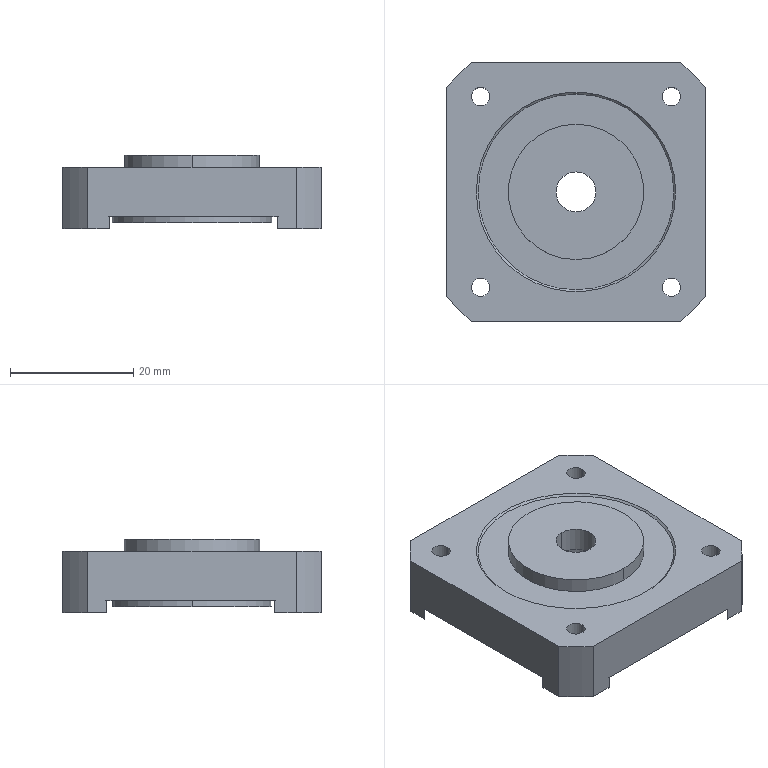Part | SolidWorks | features BaseBody 1 | 1 solid | 55 faces | box 42 x 42 x 12 mm | volume 8860 mm3 | cylinder 28 | plane 25 | cone 2 | commonest cylinder face diameters 3 x8 50.4 x4 54 x4 6.5 x2 12 x2 16 x2